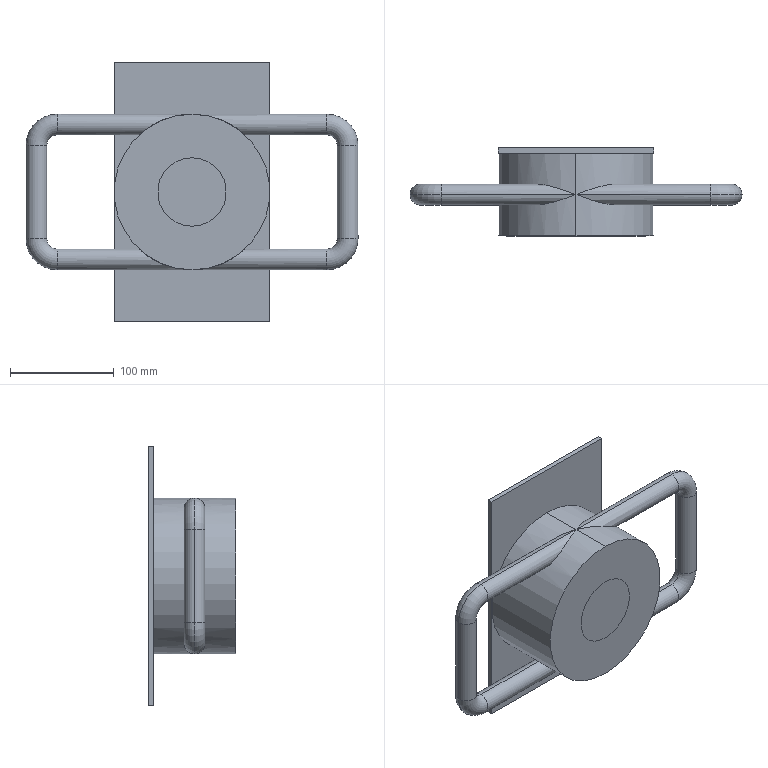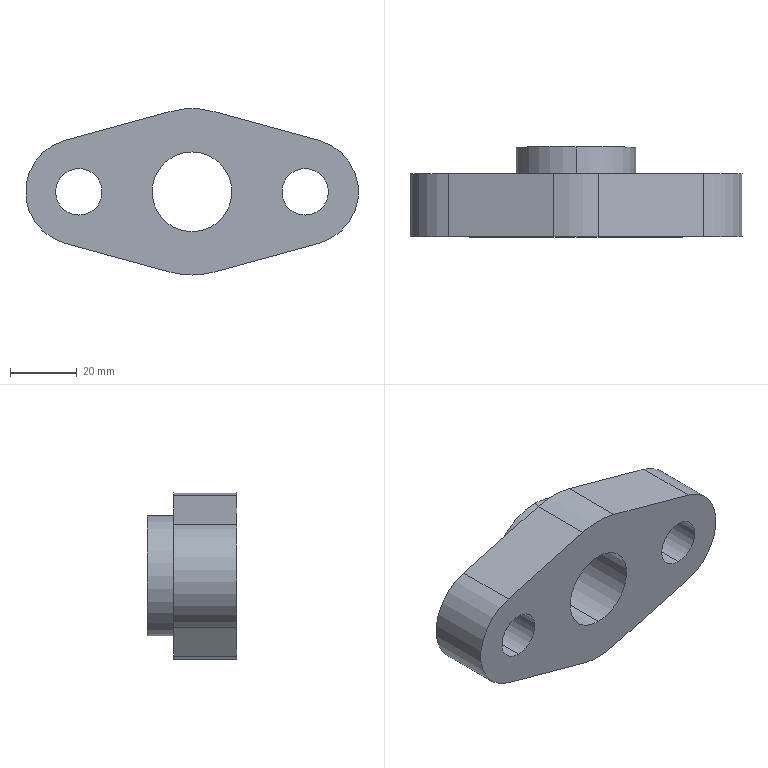Simulation study | ansys workbench
Set-up summary:
category,name,step,type,value,unit,region
solver,ansys_mapdl
solver,version,,,22.1
solver,version,,,22.1
solver,version,,,22.1
solver,version,,,22.1
units,MPA,,stated
analysis,deck1,,static,static
load_step,requested,,,1
analysis,nlgeom,,,False
mesh,nodes,,,2250
mesh,elements,,,1159
element_type,ANSYS 187 (type 1),,solid,1125
element_type,ANSYS 154 (type 2),,surface,34
load,load commands in deck,,count,1
bc,support commands in deck,,count,3
named_set,_DISPZEROUX,,component
named_set,_DISPZEROUY,,component
named_set,_DISPZEROUZ,,component
analysis,deck2,,static,static
load_step,requested,,,1
analysis,nlgeom,,,False
mesh,nodes,,,4879
mesh,elements,,,3434
element_type,ANSYS 187 (type 1),,solid,300
element_type,ANSYS 187 (type 2),,solid,475
element_type,ANSYS 187 (type 3),,solid,1623
element_type,ANSYS 174 (type 4),,contact,15
element_type,ANSYS 170 (type 5),,target,15
element_type,ANSYS 174 (type 6),,contact,154
element_type,ANSYS 170 (type 7),,target,154
element_type,ANSYS 174 (type 8),,contact,297
element_type,ANSYS 170 (type 9),,target,297
element_type,ANSYS 154 (type 10),,surface,104
load,load commands in deck,,count,1
bc,support commands in deck,,count,3
named_set,_DISPZEROUX,,component
named_set,_DISPZEROUY,,component
named_set,_DISPZEROUZ,,component
analysis,deck3,,transient,transient
load_step,requested,,,1
analysis,nlgeom,,,False
mesh,nodes,,,4879
mesh,elements,,,3330
element_type,ANSYS 291 (type 1),,thermal_solid,300
element_type,ANSYS 291 (type 2),,thermal_solid,475
element_type,ANSYS 291 (type 3),,thermal_solid,1623
element_type,ANSYS 174 (type 4),,contact,15
element_type,ANSYS 170 (type 5),,target,15
element_type,ANSYS 174 (type 6),,contact,154
element_type,ANSYS 170 (type 7),,target,154
element_type,ANSYS 174 (type 8),,contact,297
element_type,ANSYS 170 (type 9),,target,297
load,load commands in deck,,count,3
bc,support commands in deck,,count,2
named_set,_CM77,,component
named_set,_CM81,,component
analysis,deck4,,modal,modal
load_step,requested,,,1
analysis,nlgeom,,,False
mesh,nodes,,,2250
mesh,elements,,,1125
element_type,ANSYS 187 (type 1),,solid,1125
load,load commands in deck,,count,0
bc,support commands in deck,,count,0
material,1,,in results
material,1,,in results
material,2,,in results
material,3,,in results
material,1,,in results
material,2,,in results
material,3,,in results
material,1,,in results
check,setup vs results,,match,34 surface effect element(s) are not in the reader's mesh and were not compared
check,setup vs results,,match,104 surface effect element(s) are not in the reader's mesh and were not compared
check,setup vs results,,match
check,setup vs results,,match
Results summary:
result,analysis,,,static
result,last_loadstep,,,1
result,primary field,,,displacement
result,reaction total,1,FX,-0.0,N
result,reaction total,1,FY,19.793,N
result,reaction total,1,FZ,0.0,N
result,mass,,,0.000115,"NMM: mm, ton, N, s, mV, mA, degC"
result,analysis,,,static
result,last_loadstep,,,1
result,primary field,,,displacement
result,reaction total,1,FX,-0.0,N
result,reaction total,1,FY,75000,N
result,reaction total,1,FZ,-1e-06,N
result,mass,,,0.0137,"NMM: mm, ton, N, s, mV, mA, degC"
result,analysis,,,static
result,last_loadstep,,,1
result,primary field,,,temperature
result,mass,,,0.0137,"NMM: mm, ton, N, s, mV, mA, degC"
result,analysis,,,modal
result,last_loadstep,,,1
result,primary field,,,displacement